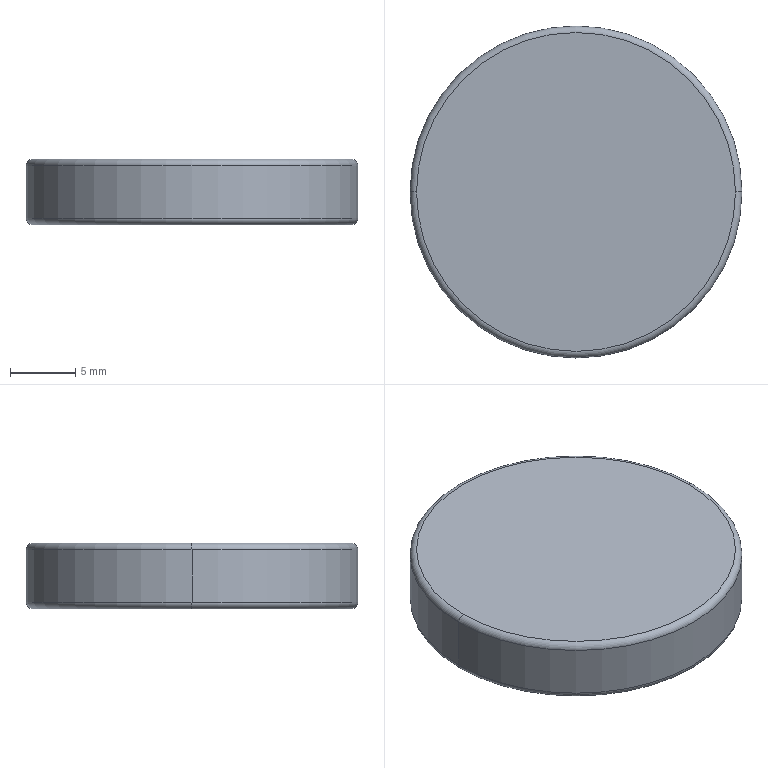Part | SolidWorks | features Extrusion 1, Fillet 1 | 1 solid | 8 faces | box 25.4 x 25.4 x 5 mm | volume 2525 mm3 | torus 4 | cylinder 2 | plane 2 | commonest cylinder face diameters 25.4 x2
STEP:
#1=CARTESIAN_POINT('',(-12.7,0.,4.5));
#2=VERTEX_POINT('',#1);
#3=CARTESIAN_POINT('',(12.7,0.,4.5));
#4=VERTEX_POINT('',#3);
#5=CARTESIAN_POINT('',(0.,0.,4.5));
#6=DIRECTION('',(0.,0.,-1.));
#7=DIRECTION('',(1.,0.,0.));
#8=AXIS2_PLACEMENT_3D('',#5,#6,#7);
#9=CIRCLE('',#8,12.7);
#10=EDGE_CURVE('',#2,#4,#9,.T.);
#11=ORIENTED_EDGE('',*,*,#10,.F.);
#12=CARTESIAN_POINT('',(-12.2,0.,5.));
#13=VERTEX_POINT('',#12);
#14=CARTESIAN_POINT('',(-12.2,0.,4.5));
#15=DIRECTION('',(0.,1.,0.));
#16=DIRECTION('',(-1.,0.,0.));
#17=AXIS2_PLACEMENT_3D('',#14,#15,#16);
#18=CIRCLE('',#17,0.5);
#19=EDGE_CURVE('',#2,#13,#18,.T.);
#20=ORIENTED_EDGE('',*,*,#19,.T.);
#21=CARTESIAN_POINT('',(12.2,0.,5.));
#22=VERTEX_POINT('',#21);
#23=CARTESIAN_POINT('',(0.,0.,5.));
#24=DIRECTION('',(0.,0.,1.));
#25=DIRECTION('',(1.,0.,0.));
#26=AXIS2_PLACEMENT_3D('',#23,#24,#25);
#27=CIRCLE('',#26,12.2);
#28=EDGE_CURVE('',#22,#13,#27,.T.);
#29=ORIENTED_EDGE('',*,*,#28,.F.);
#30=CARTESIAN_POINT('',(12.2,0.,4.5));
#31=DIRECTION('',(0.,-1.,0.));
#32=DIRECTION('',(0.,0.,-1.));
#33=AXIS2_PLACEMENT_3D('',#30,#31,#32);
#34=CIRCLE('',#33,0.5);
#35=EDGE_CURVE('',#4,#22,#34,.T.);
#36=ORIENTED_EDGE('',*,*,#35,.F.);
#37=EDGE_LOOP('',(#11,#20,#29,#36));
#38=FACE_OUTER_BOUND('',#37,.T.);
#39=CARTESIAN_POINT('',(0.,0.,4.5));
#40=DIRECTION('',(0.,0.,1.));
#41=DIRECTION('',(1.,0.,0.));
#42=AXIS2_PLACEMENT_3D('',#39,#40,#41);
#43=TOROIDAL_SURFACE('',#42,12.2,0.5);
#44=ADVANCED_FACE('',(#38),#43,.T.);
#45=CARTESIAN_POINT('',(-12.2,0.,0.));
#46=VERTEX_POINT('',#45);
#47=CARTESIAN_POINT('',(12.2,0.,0.));
#48=VERTEX_POINT('',#47);
#49=CARTESIAN_POINT('',(0.,0.,0.));
#50=DIRECTION('',(0.,0.,-1.));
#51=DIRECTION('',(1.,0.,0.));
#52=AXIS2_PLACEMENT_3D('',#49,#50,#51);
#53=CIRCLE('',#52,12.2);
#54=EDGE_CURVE('',#46,#48,#53,.T.);
#55=ORIENTED_EDGE('',*,*,#54,.F.);
#56=CARTESIAN_POINT('',(-12.7,0.,0.5));
#57=VERTEX_POINT('',#56);
#58=CARTESIAN_POINT('',(-12.2,0.,0.5));
#59=DIRECTION('',(0.,1.,0.));
#60=DIRECTION('',(-1.,0.,0.));
#61=AXIS2_PLACEMENT_3D('',#58,#59,#60);
#62=CIRCLE('',#61,0.5);
#63=EDGE_CURVE('',#46,#57,#62,.T.);
#64=ORIENTED_EDGE('',*,*,#63,.T.);
#65=CARTESIAN_POINT('',(12.7,0.,0.5));
#66=VERTEX_POINT('',#65);
#67=CARTESIAN_POINT('',(0.,0.,0.5));
#68=DIRECTION('',(0.,0.,1.));
#69=DIRECTION('',(1.,0.,0.));
#70=AXIS2_PLACEMENT_3D('',#67,#68,#69);
#71=CIRCLE('',#70,12.7);
#72=EDGE_CURVE('',#66,#57,#71,.T.);
#73=ORIENTED_EDGE('',*,*,#72,.F.);
#74=CARTESIAN_POINT('',(12.2,0.,0.5));
#75=DIRECTION('',(0.,-1.,0.));
#76=DIRECTION('',(0.,0.,-1.));
#77=AXIS2_PLACEMENT_3D('',#74,#75,#76);
#78=CIRCLE('',#77,0.5);
#79=EDGE_CURVE('',#48,#66,#78,.T.);
#80=ORIENTED_EDGE('',*,*,#79,.F.);
#81=EDGE_LOOP('',(#55,#64,#73,#80));
#82=FACE_OUTER_BOUND('',#81,.T.);
#83=CARTESIAN_POINT('',(0.,0.,0.5));
#84=DIRECTION('',(0.,0.,1.));
#85=DIRECTION('',(1.,0.,0.));
#86=AXIS2_PLACEMENT_3D('',#83,#84,#85);
#87=TOROIDAL_SURFACE('',#86,12.2,0.5);
#88=ADVANCED_FACE('',(#82),#87,.T.);
#89=ORIENTED_EDGE('',*,*,#10,.T.);
#90=CARTESIAN_POINT('',(12.7,0.,5.));
#91=DIRECTION('',(0.,0.,-1.));
#92=VECTOR('',#91,1000.);
#93=LINE('',#90,#92);
#94=EDGE_CURVE('',#4,#66,#93,.T.);
#95=ORIENTED_EDGE('',*,*,#94,.T.);
#96=ORIENTED_EDGE('',*,*,#72,.T.);
#97=CARTESIAN_POINT('',(-12.7,0.,5.));
#98=DIRECTION('',(0.,0.,-1.));
#99=VECTOR('',#98,1000.);
#100=LINE('',#97,#99);
#101=EDGE_CURVE('',#2,#57,#100,.T.);
#102=ORIENTED_EDGE('',*,*,#101,.F.);
#103=EDGE_LOOP('',(#89,#95,#96,#102));
#104=FACE_OUTER_BOUND('',#103,.T.);
#105=CARTESIAN_POINT('',(0.,0.,5.));
#106=DIRECTION('',(0.,0.,-1.));
#107=DIRECTION('',(-1.,0.,0.));
#108=AXIS2_PLACEMENT_3D('',#105,#106,#107);
#109=CYLINDRICAL_SURFACE('',#108,12.7);
#110=ADVANCED_FACE('',(#104),#109,.T.);
#111=ORIENTED_EDGE('',*,*,#94,.F.);
#112=CARTESIAN_POINT('',(0.,0.,4.5));
#113=DIRECTION('',(0.,0.,-1.));
#114=DIRECTION('',(1.,0.,0.));
#115=AXIS2_PLACEMENT_3D('',#112,#113,#114);
#116=CIRCLE('',#115,12.7);
#117=EDGE_CURVE('',#4,#2,#116,.T.);
#118=ORIENTED_EDGE('',*,*,#117,.T.);
#119=ORIENTED_EDGE('',*,*,#101,.T.);
#120=CARTESIAN_POINT('',(0.,0.,0.5));
#121=DIRECTION('',(0.,0.,1.));
#122=DIRECTION('',(1.,0.,0.));
#123=AXIS2_PLACEMENT_3D('',#120,#121,#122);
#124=CIRCLE('',#123,12.7);
#125=EDGE_CURVE('',#57,#66,#124,.T.);
#126=ORIENTED_EDGE('',*,*,#125,.T.);
#127=EDGE_LOOP('',(#111,#118,#119,#126));
#128=FACE_OUTER_BOUND('',#127,.T.);
#129=CARTESIAN_POINT('',(0.,0.,5.));
#130=DIRECTION('',(0.,0.,-1.));
#131=DIRECTION('',(-1.,0.,0.));
#132=AXIS2_PLACEMENT_3D('',#129,#130,#131);
#133=CYLINDRICAL_SURFACE('',#132,12.7);
#134=ADVANCED_FACE('',(#128),#133,.T.);
#135=ORIENTED_EDGE('',*,*,#28,.T.);
#136=CARTESIAN_POINT('',(0.,0.,5.));
#137=DIRECTION('',(0.,0.,1.));
#138=DIRECTION('',(1.,0.,0.));
#139=AXIS2_PLACEMENT_3D('',#136,#137,#138);
#140=CIRCLE('',#139,12.2);
#141=EDGE_CURVE('',#13,#22,#140,.T.);
#142=ORIENTED_EDGE('',*,*,#141,.T.);
#143=EDGE_LOOP('',(#135,#142));
#144=FACE_OUTER_BOUND('',#143,.T.);
#145=CARTESIAN_POINT('',(0.,0.,5.));
#146=DIRECTION('',(0.,0.,1.));
#147=DIRECTION('',(1.,0.,0.));
#148=AXIS2_PLACEMENT_3D('',#145,#146,#147);
#149=PLANE('',#148);
#150=ADVANCED_FACE('',(#144),#149,.T.);
#151=CARTESIAN_POINT('',(0.,0.,0.));
#152=DIRECTION('',(0.,0.,-1.));
#153=DIRECTION('',(1.,0.,0.));
#154=AXIS2_PLACEMENT_3D('',#151,#152,#153);
#155=CIRCLE('',#154,12.2);
#156=EDGE_CURVE('',#48,#46,#155,.T.);
#157=ORIENTED_EDGE('',*,*,#156,.T.);
#158=ORIENTED_EDGE('',*,*,#54,.T.);
#159=EDGE_LOOP('',(#157,#158));
#160=FACE_OUTER_BOUND('',#159,.T.);
#161=CARTESIAN_POINT('',(0.,0.,0.));
#162=DIRECTION('',(0.,0.,1.));
#163=DIRECTION('',(1.,0.,0.));
#164=AXIS2_PLACEMENT_3D('',#161,#162,#163);
#165=PLANE('',#164);
#166=ADVANCED_FACE('',(#160),#165,.F.);
#167=ORIENTED_EDGE('',*,*,#63,.F.);
#168=ORIENTED_EDGE('',*,*,#156,.F.);
#169=ORIENTED_EDGE('',*,*,#79,.T.);
#170=ORIENTED_EDGE('',*,*,#125,.F.);
#171=EDGE_LOOP('',(#167,#168,#169,#170));
#172=FACE_OUTER_BOUND('',#171,.T.);
#173=CARTESIAN_POINT('',(0.,0.,0.5));
#174=DIRECTION('',(0.,0.,1.));
#175=DIRECTION('',(1.,0.,0.));
#176=AXIS2_PLACEMENT_3D('',#173,#174,#175);
#177=TOROIDAL_SURFACE('',#176,12.2,0.5);
#178=ADVANCED_FACE('',(#172),#177,.T.);
#179=ORIENTED_EDGE('',*,*,#19,.F.);
#180=ORIENTED_EDGE('',*,*,#117,.F.);
#181=ORIENTED_EDGE('',*,*,#35,.T.);
#182=ORIENTED_EDGE('',*,*,#141,.F.);
#183=EDGE_LOOP('',(#179,#180,#181,#182));
#184=FACE_OUTER_BOUND('',#183,.T.);
#185=CARTESIAN_POINT('',(0.,0.,4.5));
#186=DIRECTION('',(0.,0.,1.));
#187=DIRECTION('',(1.,0.,0.));
#188=AXIS2_PLACEMENT_3D('',#185,#186,#187);
#189=TOROIDAL_SURFACE('',#188,12.2,0.5);
#190=ADVANCED_FACE('',(#184),#189,.T.);
#191=CLOSED_SHELL('',(#44,#88,#110,#134,#150,#166,#178,#190));
#192=MANIFOLD_SOLID_BREP('',#191);
#193=CARTESIAN_POINT('',(0.,0.,0.));
#194=DIRECTION('',(0.,0.,1.));
#195=DIRECTION('',(1.,0.,0.));
#196=AXIS2_PLACEMENT_3D('',#193,#194,#195);
#197=(LENGTH_UNIT()NAMED_UNIT(*)SI_UNIT(.MILLI.,.METRE.));
#198=UNCERTAINTY_MEASURE_WITH_UNIT(LENGTH_MEASURE(0.00001),#197,'','');
#199=(NAMED_UNIT(*)PLANE_ANGLE_UNIT()SI_UNIT($,.RADIAN.));
#200=(NAMED_UNIT(*)SI_UNIT($,.STERADIAN.)SOLID_ANGLE_UNIT());
#201=(GEOMETRIC_REPRESENTATION_CONTEXT(3)GLOBAL_UNCERTAINTY_ASSIGNED_CONTEXT((#198))GLOBAL_UNIT_ASSIGNED_CONTEXT((#197,#199,#200))REPRESENTATION_CONTEXT('',''));
#202=ADVANCED_BREP_SHAPE_REPRESENTATION('',(#192,#196),#201);